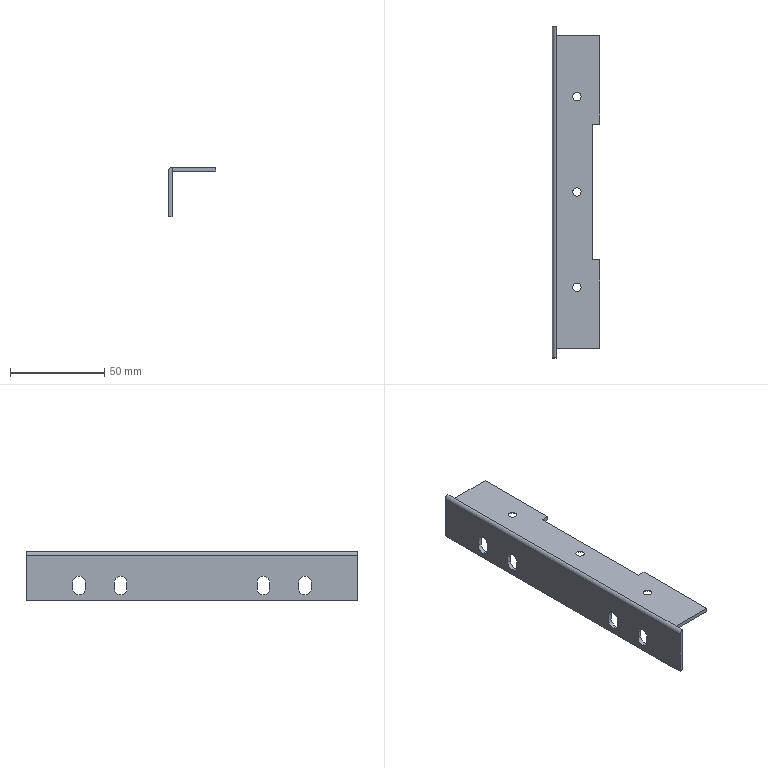Part | STEP file | Rear computer plate rib part | 1 solid | 41 faces | box 25 x 176 x 26 mm | volume 15403 mm3 | plane 22 | cylinder 13 | cone 6 | commonest cylinder face diameters 6.7 x12 4 x1